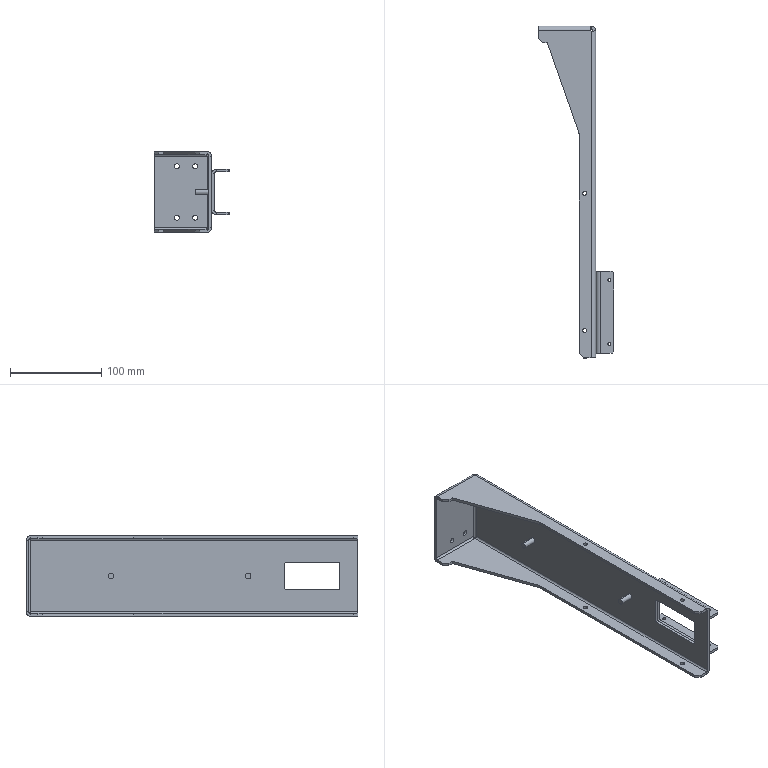Part | SolidWorks | features Chamfer 4, ICE 4, HoleWzd 3, FlatPattern 2, SMBaseFlange 2, SheetMetal 2, EdgeFlange 1 | 2 solids | 122 faces | box 83 x 363 x 88 mm | volume 165513 mm3 | plane 68 | cylinder 50 | spline 4 | commonest cylinder face diameters 4 x15 3.3 x8 4.5 x8 5.5 x8 10 x7 6 x4